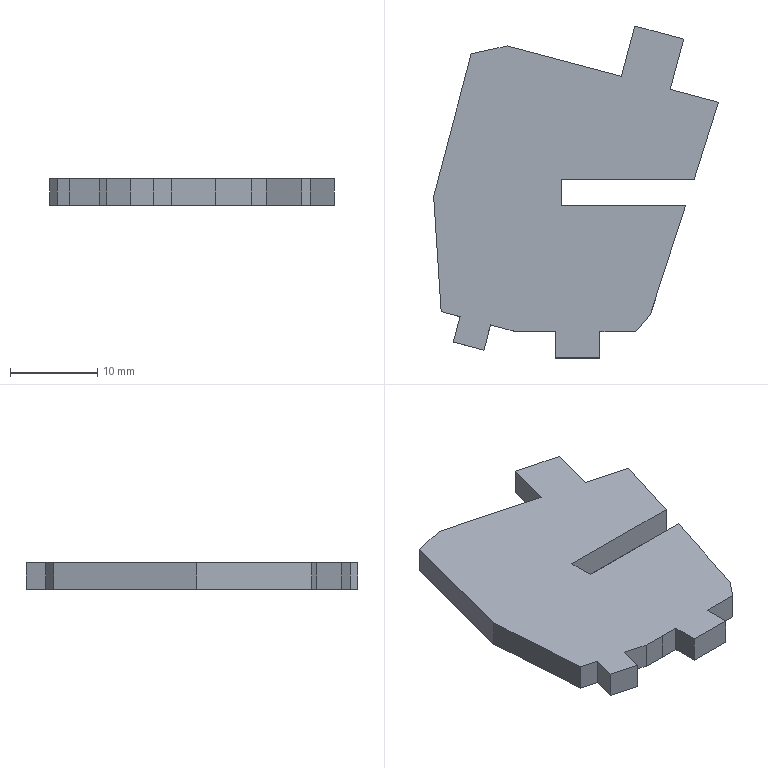Part | SolidWorks | features BaseBody 1 | 1 solid | 27 faces | box 32.712 x 38.137 x 3 mm | volume 2525 mm3 | plane 27
STEP:
#1=CARTESIAN_POINT('',(1.403,4.918,-1.5));
#2=VERTEX_POINT('',#1);
#3=CARTESIAN_POINT('',(16.692,4.918,-1.5));
#4=VERTEX_POINT('',#3);
#5=CARTESIAN_POINT('',(1.403,4.918,-1.5));
#6=DIRECTION('',(1.,0.,0.));
#7=VECTOR('',#6,1000.);
#8=LINE('',#5,#7);
#9=EDGE_CURVE('',#2,#4,#8,.T.);
#10=ORIENTED_EDGE('',*,*,#9,.F.);
#11=CARTESIAN_POINT('',(1.403,1.923,-1.5));
#12=VERTEX_POINT('',#11);
#13=CARTESIAN_POINT('',(1.403,1.923,-1.5));
#14=DIRECTION('',(0.,1.,0.));
#15=VECTOR('',#14,1000.);
#16=LINE('',#13,#15);
#17=EDGE_CURVE('',#12,#2,#16,.T.);
#18=ORIENTED_EDGE('',*,*,#17,.F.);
#19=CARTESIAN_POINT('',(15.72,1.923,-1.5));
#20=VERTEX_POINT('',#19);
#21=CARTESIAN_POINT('',(15.72,1.923,-1.5));
#22=DIRECTION('',(-1.,0.,0.));
#23=VECTOR('',#22,1000.);
#24=LINE('',#21,#23);
#25=EDGE_CURVE('',#20,#12,#24,.T.);
#26=ORIENTED_EDGE('',*,*,#25,.F.);
#27=CARTESIAN_POINT('',(11.682,-10.531,-1.5));
#28=VERTEX_POINT('',#27);
#29=CARTESIAN_POINT('',(11.682,-10.531,-1.5));
#30=DIRECTION('',(0.3085,0.9512,0.));
#31=VECTOR('',#30,1000.);
#32=LINE('',#29,#31);
#33=EDGE_CURVE('',#28,#20,#32,.T.);
#34=ORIENTED_EDGE('',*,*,#33,.F.);
#35=CARTESIAN_POINT('',(9.998,-12.584,-1.5));
#36=VERTEX_POINT('',#35);
#37=CARTESIAN_POINT('',(9.998,-12.584,-1.5));
#38=DIRECTION('',(0.6341,0.7732,0.));
#39=VECTOR('',#38,1000.);
#40=LINE('',#37,#39);
#41=EDGE_CURVE('',#36,#28,#40,.T.);
#42=ORIENTED_EDGE('',*,*,#41,.F.);
#43=CARTESIAN_POINT('',(5.866,-12.584,-1.5));
#44=VERTEX_POINT('',#43);
#45=CARTESIAN_POINT('',(5.866,-12.584,-1.5));
#46=DIRECTION('',(1.,0.,0.));
#47=VECTOR('',#46,1000.);
#48=LINE('',#45,#47);
#49=EDGE_CURVE('',#44,#36,#48,.T.);
#50=ORIENTED_EDGE('',*,*,#49,.F.);
#51=CARTESIAN_POINT('',(5.866,-15.579,-1.5));
#52=VERTEX_POINT('',#51);
#53=CARTESIAN_POINT('',(5.866,-15.579,-1.5));
#54=DIRECTION('',(0.,1.,0.));
#55=VECTOR('',#54,1000.);
#56=LINE('',#53,#55);
#57=EDGE_CURVE('',#52,#44,#56,.T.);
#58=ORIENTED_EDGE('',*,*,#57,.F.);
#59=CARTESIAN_POINT('',(0.8014,-15.579,-1.5));
#60=VERTEX_POINT('',#59);
#61=CARTESIAN_POINT('',(0.8014,-15.579,-1.5));
#62=DIRECTION('',(1.,0.,0.));
#63=VECTOR('',#62,1000.);
#64=LINE('',#61,#63);
#65=EDGE_CURVE('',#60,#52,#64,.T.);
#66=ORIENTED_EDGE('',*,*,#65,.F.);
#67=CARTESIAN_POINT('',(0.8014,-12.584,-1.5));
#68=VERTEX_POINT('',#67);
#69=CARTESIAN_POINT('',(0.8014,-12.584,-1.5));
#70=DIRECTION('',(0.,-1.,0.));
#71=VECTOR('',#70,1000.);
#72=LINE('',#69,#71);
#73=EDGE_CURVE('',#68,#60,#72,.T.);
#74=ORIENTED_EDGE('',*,*,#73,.F.);
#75=CARTESIAN_POINT('',(-1.339,-12.584,-1.5));
#76=VERTEX_POINT('',#75);
#77=CARTESIAN_POINT('',(-1.339,-12.584,-1.5));
#78=DIRECTION('',(1.,0.,0.));
#79=VECTOR('',#78,1000.);
#80=LINE('',#77,#79);
#81=EDGE_CURVE('',#76,#68,#80,.T.);
#82=ORIENTED_EDGE('',*,*,#81,.F.);
#83=CARTESIAN_POINT('',(-3.987,-12.51,-1.5));
#84=VERTEX_POINT('',#83);
#85=CARTESIAN_POINT('',(-3.987,-12.51,-1.5));
#86=DIRECTION('',(0.9996,-0.02815,0.));
#87=VECTOR('',#86,1000.);
#88=LINE('',#85,#87);
#89=EDGE_CURVE('',#84,#76,#88,.T.);
#90=ORIENTED_EDGE('',*,*,#89,.F.);
#91=CARTESIAN_POINT('',(-6.685,-11.785,-1.5));
#92=VERTEX_POINT('',#91);
#93=CARTESIAN_POINT('',(-6.685,-11.785,-1.5));
#94=DIRECTION('',(0.9658,-0.2593,0.));
#95=VECTOR('',#94,1000.);
#96=LINE('',#93,#95);
#97=EDGE_CURVE('',#92,#84,#96,.T.);
#98=ORIENTED_EDGE('',*,*,#97,.F.);
#99=CARTESIAN_POINT('',(-7.463,-14.68,-1.5));
#100=VERTEX_POINT('',#99);
#101=CARTESIAN_POINT('',(-7.463,-14.68,-1.5));
#102=DIRECTION('',(0.2595,0.9658,0.));
#103=VECTOR('',#102,1000.);
#104=LINE('',#101,#103);
#105=EDGE_CURVE('',#100,#92,#104,.T.);
#106=ORIENTED_EDGE('',*,*,#105,.F.);
#107=CARTESIAN_POINT('',(-10.961,-13.742,-1.5));
#108=VERTEX_POINT('',#107);
#109=CARTESIAN_POINT('',(-10.961,-13.742,-1.5));
#110=DIRECTION('',(0.9659,-0.2591,0.));
#111=VECTOR('',#110,1000.);
#112=LINE('',#109,#111);
#113=EDGE_CURVE('',#108,#100,#112,.T.);
#114=ORIENTED_EDGE('',*,*,#113,.F.);
#115=CARTESIAN_POINT('',(-10.185,-10.848,-1.5));
#116=VERTEX_POINT('',#115);
#117=CARTESIAN_POINT('',(-10.185,-10.848,-1.5));
#118=DIRECTION('',(-0.2591,-0.9659,0.));
#119=VECTOR('',#118,1000.);
#120=LINE('',#117,#119);
#121=EDGE_CURVE('',#116,#108,#120,.T.);
#122=ORIENTED_EDGE('',*,*,#121,.F.);
#123=CARTESIAN_POINT('',(-12.37,-10.262,-1.5));
#124=VERTEX_POINT('',#123);
#125=CARTESIAN_POINT('',(-12.37,-10.262,-1.5));
#126=DIRECTION('',(0.9659,-0.259,0.));
#127=VECTOR('',#126,1000.);
#128=LINE('',#125,#127);
#129=EDGE_CURVE('',#124,#116,#128,.T.);
#130=ORIENTED_EDGE('',*,*,#129,.F.);
#131=CARTESIAN_POINT('',(-13.232,2.968,-1.5));
#132=VERTEX_POINT('',#131);
#133=CARTESIAN_POINT('',(-13.232,2.968,-1.5));
#134=DIRECTION('',(0.065,-0.9979,0.));
#135=VECTOR('',#134,1000.);
#136=LINE('',#133,#135);
#137=EDGE_CURVE('',#132,#124,#136,.T.);
#138=ORIENTED_EDGE('',*,*,#137,.F.);
#139=CARTESIAN_POINT('',(-8.91,19.377,-1.5));
#140=VERTEX_POINT('',#139);
#141=CARTESIAN_POINT('',(-8.91,19.377,-1.5));
#142=DIRECTION('',(-0.2547,-0.967,0.));
#143=VECTOR('',#142,1000.);
#144=LINE('',#141,#143);
#145=EDGE_CURVE('',#140,#132,#144,.T.);
#146=ORIENTED_EDGE('',*,*,#145,.F.);
#147=CARTESIAN_POINT('',(-4.779,20.266,-1.5));
#148=VERTEX_POINT('',#147);
#149=CARTESIAN_POINT('',(-4.779,20.266,-1.5));
#150=DIRECTION('',(-0.9776,-0.2104,0.));
#151=VECTOR('',#150,1000.);
#152=LINE('',#149,#151);
#153=EDGE_CURVE('',#148,#140,#152,.T.);
#154=ORIENTED_EDGE('',*,*,#153,.F.);
#155=CARTESIAN_POINT('',(8.324,16.769,-1.5));
#156=VERTEX_POINT('',#155);
#157=CARTESIAN_POINT('',(8.324,16.769,-1.5));
#158=DIRECTION('',(-0.9662,0.2578,0.));
#159=VECTOR('',#158,1000.);
#160=LINE('',#157,#159);
#161=EDGE_CURVE('',#156,#148,#160,.T.);
#162=ORIENTED_EDGE('',*,*,#161,.F.);
#163=CARTESIAN_POINT('',(9.87,22.558,-1.5));
#164=VERTEX_POINT('',#163);
#165=CARTESIAN_POINT('',(9.87,22.558,-1.5));
#166=DIRECTION('',(-0.258,-0.9661,0.));
#167=VECTOR('',#166,1000.);
#168=LINE('',#165,#167);
#169=EDGE_CURVE('',#164,#156,#168,.T.);
#170=ORIENTED_EDGE('',*,*,#169,.F.);
#171=CARTESIAN_POINT('',(15.49,21.059,-1.5));
#172=VERTEX_POINT('',#171);
#173=CARTESIAN_POINT('',(15.49,21.059,-1.5));
#174=DIRECTION('',(-0.9662,0.2576,0.));
#175=VECTOR('',#174,1000.);
#176=LINE('',#173,#175);
#177=EDGE_CURVE('',#172,#164,#176,.T.);
#178=ORIENTED_EDGE('',*,*,#177,.F.);
#179=CARTESIAN_POINT('',(13.938,15.27,-1.5));
#180=VERTEX_POINT('',#179);
#181=CARTESIAN_POINT('',(13.938,15.27,-1.5));
#182=DIRECTION('',(0.259,0.9659,0.));
#183=VECTOR('',#182,1000.);
#184=LINE('',#181,#183);
#185=EDGE_CURVE('',#180,#172,#184,.T.);
#186=ORIENTED_EDGE('',*,*,#185,.F.);
#187=CARTESIAN_POINT('',(19.48,13.793,-1.5));
#188=VERTEX_POINT('',#187);
#189=CARTESIAN_POINT('',(19.48,13.793,-1.5));
#190=DIRECTION('',(-0.9662,0.2576,0.));
#191=VECTOR('',#190,1000.);
#192=LINE('',#189,#191);
#193=EDGE_CURVE('',#188,#180,#192,.T.);
#194=ORIENTED_EDGE('',*,*,#193,.F.);
#195=CARTESIAN_POINT('',(16.692,4.918,-1.5));
#196=DIRECTION('',(0.2997,0.954,0.));
#197=VECTOR('',#196,1000.);
#198=LINE('',#195,#197);
#199=EDGE_CURVE('',#4,#188,#198,.T.);
#200=ORIENTED_EDGE('',*,*,#199,.F.);
#201=EDGE_LOOP('',(#10,#18,#26,#34,#42,#50,#58,#66,#74,#82,#90,#98,#106,#114,#122,#130,#138,#146,#154,#162,#170,#178,#186,#194,#200));
#202=FACE_OUTER_BOUND('',#201,.T.);
#203=CARTESIAN_POINT('',(0.,0.,-1.5));
#204=DIRECTION('',(0.,0.,-1.));
#205=DIRECTION('',(0.,-1.,0.));
#206=AXIS2_PLACEMENT_3D('',#203,#204,#205);
#207=PLANE('',#206);
#208=ADVANCED_FACE('',(#202),#207,.T.);
#209=CARTESIAN_POINT('',(1.403,4.918,1.5));
#210=VERTEX_POINT('',#209);
#211=CARTESIAN_POINT('',(16.692,4.918,1.5));
#212=VERTEX_POINT('',#211);
#213=CARTESIAN_POINT('',(1.403,4.918,1.5));
#214=DIRECTION('',(1.,0.,0.));
#215=VECTOR('',#214,1000.);
#216=LINE('',#213,#215);
#217=EDGE_CURVE('',#210,#212,#216,.T.);
#218=ORIENTED_EDGE('',*,*,#217,.T.);
#219=CARTESIAN_POINT('',(19.48,13.793,1.5));
#220=VERTEX_POINT('',#219);
#221=CARTESIAN_POINT('',(16.692,4.918,1.5));
#222=DIRECTION('',(0.2997,0.954,0.));
#223=VECTOR('',#222,1000.);
#224=LINE('',#221,#223);
#225=EDGE_CURVE('',#212,#220,#224,.T.);
#226=ORIENTED_EDGE('',*,*,#225,.T.);
#227=CARTESIAN_POINT('',(13.938,15.27,1.5));
#228=VERTEX_POINT('',#227);
#229=CARTESIAN_POINT('',(19.48,13.793,1.5));
#230=DIRECTION('',(-0.9662,0.2576,0.));
#231=VECTOR('',#230,1000.);
#232=LINE('',#229,#231);
#233=EDGE_CURVE('',#220,#228,#232,.T.);
#234=ORIENTED_EDGE('',*,*,#233,.T.);
#235=CARTESIAN_POINT('',(15.49,21.059,1.5));
#236=VERTEX_POINT('',#235);
#237=CARTESIAN_POINT('',(13.938,15.27,1.5));
#238=DIRECTION('',(0.259,0.9659,0.));
#239=VECTOR('',#238,1000.);
#240=LINE('',#237,#239);
#241=EDGE_CURVE('',#228,#236,#240,.T.);
#242=ORIENTED_EDGE('',*,*,#241,.T.);
#243=CARTESIAN_POINT('',(9.87,22.558,1.5));
#244=VERTEX_POINT('',#243);
#245=CARTESIAN_POINT('',(15.49,21.059,1.5));
#246=DIRECTION('',(-0.9662,0.2576,0.));
#247=VECTOR('',#246,1000.);
#248=LINE('',#245,#247);
#249=EDGE_CURVE('',#236,#244,#248,.T.);
#250=ORIENTED_EDGE('',*,*,#249,.T.);
#251=CARTESIAN_POINT('',(8.324,16.769,1.5));
#252=VERTEX_POINT('',#251);
#253=CARTESIAN_POINT('',(9.87,22.558,1.5));
#254=DIRECTION('',(-0.258,-0.9661,0.));
#255=VECTOR('',#254,1000.);
#256=LINE('',#253,#255);
#257=EDGE_CURVE('',#244,#252,#256,.T.);
#258=ORIENTED_EDGE('',*,*,#257,.T.);
#259=CARTESIAN_POINT('',(-4.779,20.266,1.5));
#260=VERTEX_POINT('',#259);
#261=CARTESIAN_POINT('',(8.324,16.769,1.5));
#262=DIRECTION('',(-0.9662,0.2578,0.));
#263=VECTOR('',#262,1000.);
#264=LINE('',#261,#263);
#265=EDGE_CURVE('',#252,#260,#264,.T.);
#266=ORIENTED_EDGE('',*,*,#265,.T.);
#267=CARTESIAN_POINT('',(-8.91,19.377,1.5));
#268=VERTEX_POINT('',#267);
#269=CARTESIAN_POINT('',(-4.779,20.266,1.5));
#270=DIRECTION('',(-0.9776,-0.2104,0.));
#271=VECTOR('',#270,1000.);
#272=LINE('',#269,#271);
#273=EDGE_CURVE('',#260,#268,#272,.T.);
#274=ORIENTED_EDGE('',*,*,#273,.T.);
#275=CARTESIAN_POINT('',(-13.232,2.968,1.5));
#276=VERTEX_POINT('',#275);
#277=CARTESIAN_POINT('',(-8.91,19.377,1.5));
#278=DIRECTION('',(-0.2547,-0.967,0.));
#279=VECTOR('',#278,1000.);
#280=LINE('',#277,#279);
#281=EDGE_CURVE('',#268,#276,#280,.T.);
#282=ORIENTED_EDGE('',*,*,#281,.T.);
#283=CARTESIAN_POINT('',(-12.37,-10.262,1.5));
#284=VERTEX_POINT('',#283);
#285=CARTESIAN_POINT('',(-13.232,2.968,1.5));
#286=DIRECTION('',(0.065,-0.9979,0.));
#287=VECTOR('',#286,1000.);
#288=LINE('',#285,#287);
#289=EDGE_CURVE('',#276,#284,#288,.T.);
#290=ORIENTED_EDGE('',*,*,#289,.T.);
#291=CARTESIAN_POINT('',(-10.185,-10.848,1.5));
#292=VERTEX_POINT('',#291);
#293=CARTESIAN_POINT('',(-12.37,-10.262,1.5));
#294=DIRECTION('',(0.9659,-0.259,0.));
#295=VECTOR('',#294,1000.);
#296=LINE('',#293,#295);
#297=EDGE_CURVE('',#284,#292,#296,.T.);
#298=ORIENTED_EDGE('',*,*,#297,.T.);
#299=CARTESIAN_POINT('',(-10.961,-13.742,1.5));
#300=VERTEX_POINT('',#299);
#301=CARTESIAN_POINT('',(-10.185,-10.848,1.5));
#302=DIRECTION('',(-0.2591,-0.9659,0.));
#303=VECTOR('',#302,1000.);
#304=LINE('',#301,#303);
#305=EDGE_CURVE('',#292,#300,#304,.T.);
#306=ORIENTED_EDGE('',*,*,#305,.T.);
#307=CARTESIAN_POINT('',(-7.463,-14.68,1.5));
#308=VERTEX_POINT('',#307);
#309=CARTESIAN_POINT('',(-10.961,-13.742,1.5));
#310=DIRECTION('',(0.9659,-0.2591,0.));
#311=VECTOR('',#310,1000.);
#312=LINE('',#309,#311);
#313=EDGE_CURVE('',#300,#308,#312,.T.);
#314=ORIENTED_EDGE('',*,*,#313,.T.);
#315=CARTESIAN_POINT('',(-6.685,-11.785,1.5));
#316=VERTEX_POINT('',#315);
#317=CARTESIAN_POINT('',(-7.463,-14.68,1.5));
#318=DIRECTION('',(0.2595,0.9658,0.));
#319=VECTOR('',#318,1000.);
#320=LINE('',#317,#319);
#321=EDGE_CURVE('',#308,#316,#320,.T.);
#322=ORIENTED_EDGE('',*,*,#321,.T.);
#323=CARTESIAN_POINT('',(-3.987,-12.51,1.5));
#324=VERTEX_POINT('',#323);
#325=CARTESIAN_POINT('',(-6.685,-11.785,1.5));
#326=DIRECTION('',(0.9658,-0.2593,0.));
#327=VECTOR('',#326,1000.);
#328=LINE('',#325,#327);
#329=EDGE_CURVE('',#316,#324,#328,.T.);
#330=ORIENTED_EDGE('',*,*,#329,.T.);
#331=CARTESIAN_POINT('',(-1.339,-12.584,1.5));
#332=VERTEX_POINT('',#331);
#333=CARTESIAN_POINT('',(-3.987,-12.51,1.5));
#334=DIRECTION('',(0.9996,-0.02815,0.));
#335=VECTOR('',#334,1000.);
#336=LINE('',#333,#335);
#337=EDGE_CURVE('',#324,#332,#336,.T.);
#338=ORIENTED_EDGE('',*,*,#337,.T.);
#339=CARTESIAN_POINT('',(0.8014,-12.584,1.5));
#340=VERTEX_POINT('',#339);
#341=CARTESIAN_POINT('',(-1.339,-12.584,1.5));
#342=DIRECTION('',(1.,0.,0.));
#343=VECTOR('',#342,1000.);
#344=LINE('',#341,#343);
#345=EDGE_CURVE('',#332,#340,#344,.T.);
#346=ORIENTED_EDGE('',*,*,#345,.T.);
#347=CARTESIAN_POINT('',(0.8014,-15.579,1.5));
#348=VERTEX_POINT('',#347);
#349=CARTESIAN_POINT('',(0.8014,-12.584,1.5));
#350=DIRECTION('',(0.,-1.,0.));
#351=VECTOR('',#350,1000.);
#352=LINE('',#349,#351);
#353=EDGE_CURVE('',#340,#348,#352,.T.);
#354=ORIENTED_EDGE('',*,*,#353,.T.);
#355=CARTESIAN_POINT('',(5.866,-15.579,1.5));
#356=VERTEX_POINT('',#355);
#357=CARTESIAN_POINT('',(0.8014,-15.579,1.5));
#358=DIRECTION('',(1.,0.,0.));
#359=VECTOR('',#358,1000.);
#360=LINE('',#357,#359);
#361=EDGE_CURVE('',#348,#356,#360,.T.);
#362=ORIENTED_EDGE('',*,*,#361,.T.);
#363=CARTESIAN_POINT('',(5.866,-12.584,1.5));
#364=VERTEX_POINT('',#363);
#365=CARTESIAN_POINT('',(5.866,-15.579,1.5));
#366=DIRECTION('',(0.,1.,0.));
#367=VECTOR('',#366,1000.);
#368=LINE('',#365,#367);
#369=EDGE_CURVE('',#356,#364,#368,.T.);
#370=ORIENTED_EDGE('',*,*,#369,.T.);
#371=CARTESIAN_POINT('',(9.998,-12.584,1.5));
#372=VERTEX_POINT('',#371);
#373=CARTESIAN_POINT('',(5.866,-12.584,1.5));
#374=DIRECTION('',(1.,0.,0.));
#375=VECTOR('',#374,1000.);
#376=LINE('',#373,#375);
#377=EDGE_CURVE('',#364,#372,#376,.T.);
#378=ORIENTED_EDGE('',*,*,#377,.T.);
#379=CARTESIAN_POINT('',(11.682,-10.531,1.5));
#380=VERTEX_POINT('',#379);
#381=CARTESIAN_POINT('',(9.998,-12.584,1.5));
#382=DIRECTION('',(0.6341,0.7732,0.));
#383=VECTOR('',#382,1000.);
#384=LINE('',#381,#383);
#385=EDGE_CURVE('',#372,#380,#384,.T.);
#386=ORIENTED_EDGE('',*,*,#385,.T.);
#387=CARTESIAN_POINT('',(15.72,1.923,1.5));
#388=VERTEX_POINT('',#387);
#389=CARTESIAN_POINT('',(11.682,-10.531,1.5));
#390=DIRECTION('',(0.3085,0.9512,0.));
#391=VECTOR('',#390,1000.);
#392=LINE('',#389,#391);
#393=EDGE_CURVE('',#380,#388,#392,.T.);
#394=ORIENTED_EDGE('',*,*,#393,.T.);
#395=CARTESIAN_POINT('',(1.403,1.923,1.5));
#396=VERTEX_POINT('',#395);
#397=CARTESIAN_POINT('',(15.72,1.923,1.5));
#398=DIRECTION('',(-1.,0.,0.));
#399=VECTOR('',#398,1000.);
#400=LINE('',#397,#399);
#401=EDGE_CURVE('',#388,#396,#400,.T.);
#402=ORIENTED_EDGE('',*,*,#401,.T.);
#403=CARTESIAN_POINT('',(1.403,1.923,1.5));
#404=DIRECTION('',(0.,1.,0.));
#405=VECTOR('',#404,1000.);
#406=LINE('',#403,#405);
#407=EDGE_CURVE('',#396,#210,#406,.T.);
#408=ORIENTED_EDGE('',*,*,#407,.T.);
#409=EDGE_LOOP('',(#218,#226,#234,#242,#250,#258,#266,#274,#282,#290,#298,#306,#314,#322,#330,#338,#346,#354,#362,#370,#378,#386,#394,#402,#408));
#410=FACE_OUTER_BOUND('',#409,.T.);
#411=CARTESIAN_POINT('',(0.,0.,1.5));
#412=DIRECTION('',(0.,0.,-1.));
#413=DIRECTION('',(0.,-1.,0.));
#414=AXIS2_PLACEMENT_3D('',#411,#412,#413);
#415=PLANE('',#414);
#416=ADVANCED_FACE('',(#410),#415,.F.);
#417=ORIENTED_EDGE('',*,*,#17,.T.);
#418=CARTESIAN_POINT('',(1.403,4.918,1.5));
#419=DIRECTION('',(0.,0.,-1.));
#420=VECTOR('',#419,1000.);
#421=LINE('',#418,#420);
#422=EDGE_CURVE('',#210,#2,#421,.T.);
#423=ORIENTED_EDGE('',*,*,#422,.F.);
#424=ORIENTED_EDGE('',*,*,#407,.F.);
#425=CARTESIAN_POINT('',(1.403,1.923,1.5));
#426=DIRECTION('',(0.,0.,-1.));
#427=VECTOR('',#426,1000.);
#428=LINE('',#425,#427);
#429=EDGE_CURVE('',#396,#12,#428,.T.);
#430=ORIENTED_EDGE('',*,*,#429,.T.);
#431=EDGE_LOOP('',(#417,#423,#424,#430));
#432=FACE_OUTER_BOUND('',#431,.T.);
#433=CARTESIAN_POINT('',(1.403,1.923,1.5));
#434=DIRECTION('',(-1.,0.,0.));
#435=DIRECTION('',(0.,0.,1.));
#436=AXIS2_PLACEMENT_3D('',#433,#434,#435);
#437=PLANE('',#436);
#438=ADVANCED_FACE('',(#432),#437,.F.);
#439=ORIENTED_EDGE('',*,*,#25,.T.);
#440=ORIENTED_EDGE('',*,*,#429,.F.);
#441=ORIENTED_EDGE('',*,*,#401,.F.);
#442=CARTESIAN_POINT('',(15.72,1.923,1.5));
#443=DIRECTION('',(0.,0.,-1.));
#444=VECTOR('',#443,1000.);
#445=LINE('',#442,#444);
#446=EDGE_CURVE('',#388,#20,#445,.T.);
#447=ORIENTED_EDGE('',*,*,#446,.T.);
#448=EDGE_LOOP('',(#439,#440,#441,#447));
#449=FACE_OUTER_BOUND('',#448,.T.);
#450=CARTESIAN_POINT('',(15.72,1.923,1.5));
#451=DIRECTION('',(0.,-1.,0.));
#452=DIRECTION('',(0.,0.,-1.));
#453=AXIS2_PLACEMENT_3D('',#450,#451,#452);
#454=PLANE('',#453);
#455=ADVANCED_FACE('',(#449),#454,.F.);
#456=ORIENTED_EDGE('',*,*,#33,.T.);
#457=ORIENTED_EDGE('',*,*,#446,.F.);
#458=ORIENTED_EDGE('',*,*,#393,.F.);
#459=CARTESIAN_POINT('',(11.682,-10.531,1.5));
#460=DIRECTION('',(0.,0.,-1.));
#461=VECTOR('',#460,1000.);
#462=LINE('',#459,#461);
#463=EDGE_CURVE('',#380,#28,#462,.T.);
#464=ORIENTED_EDGE('',*,*,#463,.T.);
#465=EDGE_LOOP('',(#456,#457,#458,#464));
#466=FACE_OUTER_BOUND('',#465,.T.);
#467=CARTESIAN_POINT('',(11.682,-10.531,1.5));
#468=DIRECTION('',(-0.9512,0.3085,0.));
#469=DIRECTION('',(0.,0.,1.));
#470=AXIS2_PLACEMENT_3D('',#467,#468,#469);
#471=PLANE('',#470);
#472=ADVANCED_FACE('',(#466),#471,.F.);
#473=ORIENTED_EDGE('',*,*,#41,.T.);
#474=ORIENTED_EDGE('',*,*,#463,.F.);
#475=ORIENTED_EDGE('',*,*,#385,.F.);
#476=CARTESIAN_POINT('',(9.998,-12.584,1.5));
#477=DIRECTION('',(0.,0.,-1.));
#478=VECTOR('',#477,1000.);
#479=LINE('',#476,#478);
#480=EDGE_CURVE('',#372,#36,#479,.T.);
#481=ORIENTED_EDGE('',*,*,#480,.T.);
#482=EDGE_LOOP('',(#473,#474,#475,#481));
#483=FACE_OUTER_BOUND('',#482,.T.);
#484=CARTESIAN_POINT('',(9.998,-12.584,1.5));
#485=DIRECTION('',(-0.7732,0.6341,0.));
#486=DIRECTION('',(0.,0.,1.));
#487=AXIS2_PLACEMENT_3D('',#484,#485,#486);
#488=PLANE('',#487);
#489=ADVANCED_FACE('',(#483),#488,.F.);
#490=ORIENTED_EDGE('',*,*,#49,.T.);
#491=ORIENTED_EDGE('',*,*,#480,.F.);
#492=ORIENTED_EDGE('',*,*,#377,.F.);
#493=CARTESIAN_POINT('',(5.866,-12.584,1.5));
#494=DIRECTION('',(0.,0.,-1.));
#495=VECTOR('',#494,1000.);
#496=LINE('',#493,#495);
#497=EDGE_CURVE('',#364,#44,#496,.T.);
#498=ORIENTED_EDGE('',*,*,#497,.T.);
#499=EDGE_LOOP('',(#490,#491,#492,#498));
#500=FACE_OUTER_BOUND('',#499,.T.);
#501=CARTESIAN_POINT('',(5.866,-12.584,1.5));
#502=DIRECTION('',(0.,1.,0.));
#503=DIRECTION('',(1.,0.,0.));
#504=AXIS2_PLACEMENT_3D('',#501,#502,#503);
#505=PLANE('',#504);
#506=ADVANCED_FACE('',(#500),#505,.F.);
#507=ORIENTED_EDGE('',*,*,#57,.T.);
#508=ORIENTED_EDGE('',*,*,#497,.F.);
#509=ORIENTED_EDGE('',*,*,#369,.F.);
#510=CARTESIAN_POINT('',(5.866,-15.579,1.5));
#511=DIRECTION('',(0.,0.,-1.));
#512=VECTOR('',#511,1000.);
#513=LINE('',#510,#512);
#514=EDGE_CURVE('',#356,#52,#513,.T.);
#515=ORIENTED_EDGE('',*,*,#514,.T.);
#516=EDGE_LOOP('',(#507,#508,#509,#515));
#517=FACE_OUTER_BOUND('',#516,.T.);
#518=CARTESIAN_POINT('',(5.866,-15.579,1.5));
#519=DIRECTION('',(-1.,0.,0.));
#520=DIRECTION('',(0.,0.,1.));
#521=AXIS2_PLACEMENT_3D('',#518,#519,#520);
#522=PLANE('',#521);
#523=ADVANCED_FACE('',(#517),#522,.F.);
#524=ORIENTED_EDGE('',*,*,#65,.T.);
#525=ORIENTED_EDGE('',*,*,#514,.F.);
#526=ORIENTED_EDGE('',*,*,#361,.F.);
#527=CARTESIAN_POINT('',(0.8014,-15.579,1.5));
#528=DIRECTION('',(0.,0.,-1.));
#529=VECTOR('',#528,1000.);
#530=LINE('',#527,#529);
#531=EDGE_CURVE('',#348,#60,#530,.T.);
#532=ORIENTED_EDGE('',*,*,#531,.T.);
#533=EDGE_LOOP('',(#524,#525,#526,#532));
#534=FACE_OUTER_BOUND('',#533,.T.);
#535=CARTESIAN_POINT('',(0.8014,-15.579,1.5));
#536=DIRECTION('',(0.,1.,0.));
#537=DIRECTION('',(1.,0.,0.));
#538=AXIS2_PLACEMENT_3D('',#535,#536,#537);
#539=PLANE('',#538);
#540=ADVANCED_FACE('',(#534),#539,.F.);
#541=ORIENTED_EDGE('',*,*,#73,.T.);
#542=ORIENTED_EDGE('',*,*,#531,.F.);
#543=ORIENTED_EDGE('',*,*,#353,.F.);
#544=CARTESIAN_POINT('',(0.8014,-12.584,1.5));
#545=DIRECTION('',(0.,0.,-1.));
#546=VECTOR('',#545,1000.);
#547=LINE('',#544,#546);
#548=EDGE_CURVE('',#340,#68,#547,.T.);
#549=ORIENTED_EDGE('',*,*,#548,.T.);
#550=EDGE_LOOP('',(#541,#542,#543,#549));
#551=FACE_OUTER_BOUND('',#550,.T.);
#552=CARTESIAN_POINT('',(0.8014,-12.584,1.5));
#553=DIRECTION('',(1.,0.,0.));
#554=DIRECTION('',(0.,1.,0.));
#555=AXIS2_PLACEMENT_3D('',#552,#553,#554);
#556=PLANE('',#555);
#557=ADVANCED_FACE('',(#551),#556,.F.);
#558=ORIENTED_EDGE('',*,*,#81,.T.);
#559=ORIENTED_EDGE('',*,*,#548,.F.);
#560=ORIENTED_EDGE('',*,*,#345,.F.);
#561=CARTESIAN_POINT('',(-1.339,-12.584,1.5));
#562=DIRECTION('',(0.,0.,-1.));
#563=VECTOR('',#562,1000.);
#564=LINE('',#561,#563);
#565=EDGE_CURVE('',#332,#76,#564,.T.);
#566=ORIENTED_EDGE('',*,*,#565,.T.);
#567=EDGE_LOOP('',(#558,#559,#560,#566));
#568=FACE_OUTER_BOUND('',#567,.T.);
#569=CARTESIAN_POINT('',(-1.339,-12.584,1.5));
#570=DIRECTION('',(0.,1.,0.));
#571=DIRECTION('',(1.,0.,0.));
#572=AXIS2_PLACEMENT_3D('',#569,#570,#571);
#573=PLANE('',#572);
#574=ADVANCED_FACE('',(#568),#573,.F.);
#575=ORIENTED_EDGE('',*,*,#89,.T.);
#576=ORIENTED_EDGE('',*,*,#565,.F.);
#577=ORIENTED_EDGE('',*,*,#337,.F.);
#578=CARTESIAN_POINT('',(-3.987,-12.51,1.5));
#579=DIRECTION('',(0.,0.,-1.));
#580=VECTOR('',#579,1000.);
#581=LINE('',#578,#580);
#582=EDGE_CURVE('',#324,#84,#581,.T.);
#583=ORIENTED_EDGE('',*,*,#582,.T.);
#584=EDGE_LOOP('',(#575,#576,#577,#583));
#585=FACE_OUTER_BOUND('',#584,.T.);
#586=CARTESIAN_POINT('',(-3.987,-12.51,1.5));
#587=DIRECTION('',(0.02815,0.9996,0.));
#588=DIRECTION('',(0.,0.,-1.));
#589=AXIS2_PLACEMENT_3D('',#586,#587,#588);
#590=PLANE('',#589);
#591=ADVANCED_FACE('',(#585),#590,.F.);
#592=ORIENTED_EDGE('',*,*,#97,.T.);
#593=ORIENTED_EDGE('',*,*,#582,.F.);
#594=ORIENTED_EDGE('',*,*,#329,.F.);
#595=CARTESIAN_POINT('',(-6.685,-11.785,1.5));
#596=DIRECTION('',(0.,0.,-1.));
#597=VECTOR('',#596,1000.);
#598=LINE('',#595,#597);
#599=EDGE_CURVE('',#316,#92,#598,.T.);
#600=ORIENTED_EDGE('',*,*,#599,.T.);
#601=EDGE_LOOP('',(#592,#593,#594,#600));
#602=FACE_OUTER_BOUND('',#601,.T.);
#603=CARTESIAN_POINT('',(-6.685,-11.785,1.5));
#604=DIRECTION('',(0.2593,0.9658,0.));
#605=DIRECTION('',(0.,0.,-1.));
#606=AXIS2_PLACEMENT_3D('',#603,#604,#605);
#607=PLANE('',#606);
#608=ADVANCED_FACE('',(#602),#607,.F.);
#609=ORIENTED_EDGE('',*,*,#105,.T.);
#610=ORIENTED_EDGE('',*,*,#599,.F.);
#611=ORIENTED_EDGE('',*,*,#321,.F.);
#612=CARTESIAN_POINT('',(-7.463,-14.68,1.5));
#613=DIRECTION('',(0.,0.,-1.));
#614=VECTOR('',#613,1000.);
#615=LINE('',#612,#614);
#616=EDGE_CURVE('',#308,#100,#615,.T.);
#617=ORIENTED_EDGE('',*,*,#616,.T.);
#618=EDGE_LOOP('',(#609,#610,#611,#617));
#619=FACE_OUTER_BOUND('',#618,.T.);
#620=CARTESIAN_POINT('',(-7.463,-14.68,1.5));
#621=DIRECTION('',(-0.9658,0.2595,0.));
#622=DIRECTION('',(0.,0.,1.));
#623=AXIS2_PLACEMENT_3D('',#620,#621,#622);
#624=PLANE('',#623);
#625=ADVANCED_FACE('',(#619),#624,.F.);
#626=ORIENTED_EDGE('',*,*,#113,.T.);
#627=ORIENTED_EDGE('',*,*,#616,.F.);
#628=ORIENTED_EDGE('',*,*,#313,.F.);
#629=CARTESIAN_POINT('',(-10.961,-13.742,1.5));
#630=DIRECTION('',(0.,0.,-1.));
#631=VECTOR('',#630,1000.);
#632=LINE('',#629,#631);
#633=EDGE_CURVE('',#300,#108,#632,.T.);
#634=ORIENTED_EDGE('',*,*,#633,.T.);
#635=EDGE_LOOP('',(#626,#627,#628,#634));
#636=FACE_OUTER_BOUND('',#635,.T.);
#637=CARTESIAN_POINT('',(-10.961,-13.742,1.5));
#638=DIRECTION('',(0.2591,0.9659,0.));
#639=DIRECTION('',(0.,0.,-1.));
#640=AXIS2_PLACEMENT_3D('',#637,#638,#639);
#641=PLANE('',#640);
#642=ADVANCED_FACE('',(#636),#641,.F.);
#643=ORIENTED_EDGE('',*,*,#121,.T.);
#644=ORIENTED_EDGE('',*,*,#633,.F.);
#645=ORIENTED_EDGE('',*,*,#305,.F.);
#646=CARTESIAN_POINT('',(-10.185,-10.848,1.5));
#647=DIRECTION('',(0.,0.,-1.));
#648=VECTOR('',#647,1000.);
#649=LINE('',#646,#648);
#650=EDGE_CURVE('',#292,#116,#649,.T.);
#651=ORIENTED_EDGE('',*,*,#650,.T.);
#652=EDGE_LOOP('',(#643,#644,#645,#651));
#653=FACE_OUTER_BOUND('',#652,.T.);
#654=CARTESIAN_POINT('',(-10.185,-10.848,1.5));
#655=DIRECTION('',(0.9659,-0.2591,0.));
#656=DIRECTION('',(0.,0.,-1.));
#657=AXIS2_PLACEMENT_3D('',#654,#655,#656);
#658=PLANE('',#657);
#659=ADVANCED_FACE('',(#653),#658,.F.);
#660=ORIENTED_EDGE('',*,*,#129,.T.);
#661=ORIENTED_EDGE('',*,*,#650,.F.);
#662=ORIENTED_EDGE('',*,*,#297,.F.);
#663=CARTESIAN_POINT('',(-12.37,-10.262,1.5));
#664=DIRECTION('',(0.,0.,-1.));
#665=VECTOR('',#664,1000.);
#666=LINE('',#663,#665);
#667=EDGE_CURVE('',#284,#124,#666,.T.);
#668=ORIENTED_EDGE('',*,*,#667,.T.);
#669=EDGE_LOOP('',(#660,#661,#662,#668));
#670=FACE_OUTER_BOUND('',#669,.T.);
#671=CARTESIAN_POINT('',(-12.37,-10.262,1.5));
#672=DIRECTION('',(0.259,0.9659,0.));
#673=DIRECTION('',(0.,0.,-1.));
#674=AXIS2_PLACEMENT_3D('',#671,#672,#673);
#675=PLANE('',#674);
#676=ADVANCED_FACE('',(#670),#675,.F.);
#677=ORIENTED_EDGE('',*,*,#137,.T.);
#678=ORIENTED_EDGE('',*,*,#667,.F.);
#679=ORIENTED_EDGE('',*,*,#289,.F.);
#680=CARTESIAN_POINT('',(-13.232,2.968,1.5));
#681=DIRECTION('',(0.,0.,-1.));
#682=VECTOR('',#681,1000.);
#683=LINE('',#680,#682);
#684=EDGE_CURVE('',#276,#132,#683,.T.);
#685=ORIENTED_EDGE('',*,*,#684,.T.);
#686=EDGE_LOOP('',(#677,#678,#679,#685));
#687=FACE_OUTER_BOUND('',#686,.T.);
#688=CARTESIAN_POINT('',(-13.232,2.968,1.5));
#689=DIRECTION('',(0.9979,0.065,0.));
#690=DIRECTION('',(0.,0.,-1.));
#691=AXIS2_PLACEMENT_3D('',#688,#689,#690);
#692=PLANE('',#691);
#693=ADVANCED_FACE('',(#687),#692,.F.);
#694=ORIENTED_EDGE('',*,*,#145,.T.);
#695=ORIENTED_EDGE('',*,*,#684,.F.);
#696=ORIENTED_EDGE('',*,*,#281,.F.);
#697=CARTESIAN_POINT('',(-8.91,19.377,1.5));
#698=DIRECTION('',(0.,0.,-1.));
#699=VECTOR('',#698,1000.);
#700=LINE('',#697,#699);
#701=EDGE_CURVE('',#268,#140,#700,.T.);
#702=ORIENTED_EDGE('',*,*,#701,.T.);
#703=EDGE_LOOP('',(#694,#695,#696,#702));
#704=FACE_OUTER_BOUND('',#703,.T.);
#705=CARTESIAN_POINT('',(-8.91,19.377,1.5));
#706=DIRECTION('',(0.967,-0.2547,0.));
#707=DIRECTION('',(0.,0.,-1.));
#708=AXIS2_PLACEMENT_3D('',#705,#706,#707);
#709=PLANE('',#708);
#710=ADVANCED_FACE('',(#704),#709,.F.);
#711=ORIENTED_EDGE('',*,*,#153,.T.);
#712=ORIENTED_EDGE('',*,*,#701,.F.);
#713=ORIENTED_EDGE('',*,*,#273,.F.);
#714=CARTESIAN_POINT('',(-4.779,20.266,1.5));
#715=DIRECTION('',(0.,0.,-1.));
#716=VECTOR('',#715,1000.);
#717=LINE('',#714,#716);
#718=EDGE_CURVE('',#260,#148,#717,.T.);
#719=ORIENTED_EDGE('',*,*,#718,.T.);
#720=EDGE_LOOP('',(#711,#712,#713,#719));
#721=FACE_OUTER_BOUND('',#720,.T.);
#722=CARTESIAN_POINT('',(-4.779,20.266,1.5));
#723=DIRECTION('',(0.2104,-0.9776,0.));
#724=DIRECTION('',(0.,0.,-1.));
#725=AXIS2_PLACEMENT_3D('',#722,#723,#724);
#726=PLANE('',#725);
#727=ADVANCED_FACE('',(#721),#726,.F.);
#728=ORIENTED_EDGE('',*,*,#161,.T.);
#729=ORIENTED_EDGE('',*,*,#718,.F.);
#730=ORIENTED_EDGE('',*,*,#265,.F.);
#731=CARTESIAN_POINT('',(8.324,16.769,1.5));
#732=DIRECTION('',(0.,0.,-1.));
#733=VECTOR('',#732,1000.);
#734=LINE('',#731,#733);
#735=EDGE_CURVE('',#252,#156,#734,.T.);
#736=ORIENTED_EDGE('',*,*,#735,.T.);
#737=EDGE_LOOP('',(#728,#729,#730,#736));
#738=FACE_OUTER_BOUND('',#737,.T.);
#739=CARTESIAN_POINT('',(8.324,16.769,1.5));
#740=DIRECTION('',(-0.2578,-0.9662,0.));
#741=DIRECTION('',(-0.9662,0.2578,0.));
#742=AXIS2_PLACEMENT_3D('',#739,#740,#741);
#743=PLANE('',#742);
#744=ADVANCED_FACE('',(#738),#743,.F.);
#745=ORIENTED_EDGE('',*,*,#169,.T.);
#746=ORIENTED_EDGE('',*,*,#735,.F.);
#747=ORIENTED_EDGE('',*,*,#257,.F.);
#748=CARTESIAN_POINT('',(9.87,22.558,1.5));
#749=DIRECTION('',(0.,0.,-1.));
#750=VECTOR('',#749,1000.);
#751=LINE('',#748,#750);
#752=EDGE_CURVE('',#244,#164,#751,.T.);
#753=ORIENTED_EDGE('',*,*,#752,.T.);
#754=EDGE_LOOP('',(#745,#746,#747,#753));
#755=FACE_OUTER_BOUND('',#754,.T.);
#756=CARTESIAN_POINT('',(9.87,22.558,1.5));
#757=DIRECTION('',(0.9661,-0.258,0.));
#758=DIRECTION('',(0.,0.,-1.));
#759=AXIS2_PLACEMENT_3D('',#756,#757,#758);
#760=PLANE('',#759);
#761=ADVANCED_FACE('',(#755),#760,.F.);
#762=ORIENTED_EDGE('',*,*,#177,.T.);
#763=ORIENTED_EDGE('',*,*,#752,.F.);
#764=ORIENTED_EDGE('',*,*,#249,.F.);
#765=CARTESIAN_POINT('',(15.49,21.059,1.5));
#766=DIRECTION('',(0.,0.,-1.));
#767=VECTOR('',#766,1000.);
#768=LINE('',#765,#767);
#769=EDGE_CURVE('',#236,#172,#768,.T.);
#770=ORIENTED_EDGE('',*,*,#769,.T.);
#771=EDGE_LOOP('',(#762,#763,#764,#770));
#772=FACE_OUTER_BOUND('',#771,.T.);
#773=CARTESIAN_POINT('',(15.49,21.059,1.5));
#774=DIRECTION('',(-0.2576,-0.9662,0.));
#775=DIRECTION('',(-0.9662,0.2576,0.));
#776=AXIS2_PLACEMENT_3D('',#773,#774,#775);
#777=PLANE('',#776);
#778=ADVANCED_FACE('',(#772),#777,.F.);
#779=ORIENTED_EDGE('',*,*,#185,.T.);
#780=ORIENTED_EDGE('',*,*,#769,.F.);
#781=ORIENTED_EDGE('',*,*,#241,.F.);
#782=CARTESIAN_POINT('',(13.938,15.27,1.5));
#783=DIRECTION('',(0.,0.,-1.));
#784=VECTOR('',#783,1000.);
#785=LINE('',#782,#784);
#786=EDGE_CURVE('',#228,#180,#785,.T.);
#787=ORIENTED_EDGE('',*,*,#786,.T.);
#788=EDGE_LOOP('',(#779,#780,#781,#787));
#789=FACE_OUTER_BOUND('',#788,.T.);
#790=CARTESIAN_POINT('',(13.938,15.27,1.5));
#791=DIRECTION('',(-0.9659,0.259,0.));
#792=DIRECTION('',(0.,0.,1.));
#793=AXIS2_PLACEMENT_3D('',#790,#791,#792);
#794=PLANE('',#793);
#795=ADVANCED_FACE('',(#789),#794,.F.);
#796=ORIENTED_EDGE('',*,*,#193,.T.);
#797=ORIENTED_EDGE('',*,*,#786,.F.);
#798=ORIENTED_EDGE('',*,*,#233,.F.);
#799=CARTESIAN_POINT('',(19.48,13.793,1.5));
#800=DIRECTION('',(0.,0.,-1.));
#801=VECTOR('',#800,1000.);
#802=LINE('',#799,#801);
#803=EDGE_CURVE('',#220,#188,#802,.T.);
#804=ORIENTED_EDGE('',*,*,#803,.T.);
#805=EDGE_LOOP('',(#796,#797,#798,#804));
#806=FACE_OUTER_BOUND('',#805,.T.);
#807=CARTESIAN_POINT('',(19.48,13.793,1.5));
#808=DIRECTION('',(-0.2576,-0.9662,0.));
#809=DIRECTION('',(-0.9662,0.2576,0.));
#810=AXIS2_PLACEMENT_3D('',#807,#808,#809);
#811=PLANE('',#810);
#812=ADVANCED_FACE('',(#806),#811,.F.);
#813=ORIENTED_EDGE('',*,*,#199,.T.);
#814=ORIENTED_EDGE('',*,*,#803,.F.);
#815=ORIENTED_EDGE('',*,*,#225,.F.);
#816=CARTESIAN_POINT('',(16.692,4.918,1.5));
#817=DIRECTION('',(0.,0.,-1.));
#818=VECTOR('',#817,1000.);
#819=LINE('',#816,#818);
#820=EDGE_CURVE('',#212,#4,#819,.T.);
#821=ORIENTED_EDGE('',*,*,#820,.T.);
#822=EDGE_LOOP('',(#813,#814,#815,#821));
#823=FACE_OUTER_BOUND('',#822,.T.);
#824=CARTESIAN_POINT('',(16.692,4.918,1.5));
#825=DIRECTION('',(-0.954,0.2997,0.));
#826=DIRECTION('',(0.,0.,1.));
#827=AXIS2_PLACEMENT_3D('',#824,#825,#826);
#828=PLANE('',#827);
#829=ADVANCED_FACE('',(#823),#828,.F.);
#830=ORIENTED_EDGE('',*,*,#9,.T.);
#831=ORIENTED_EDGE('',*,*,#820,.F.);
#832=ORIENTED_EDGE('',*,*,#217,.F.);
#833=ORIENTED_EDGE('',*,*,#422,.T.);
#834=EDGE_LOOP('',(#830,#831,#832,#833));
#835=FACE_OUTER_BOUND('',#834,.T.);
#836=CARTESIAN_POINT('',(1.403,4.918,1.5));
#837=DIRECTION('',(0.,1.,0.));
#838=DIRECTION('',(1.,0.,0.));
#839=AXIS2_PLACEMENT_3D('',#836,#837,#838);
#840=PLANE('',#839);
#841=ADVANCED_FACE('',(#835),#840,.F.);
#842=CLOSED_SHELL('',(#208,#416,#438,#455,#472,#489,#506,#523,#540,#557,#574,#591,#608,#625,#642,#659,#676,#693,#710,#727,#744,#761,#778,#795,#812,#829,#841));
#843=MANIFOLD_SOLID_BREP('',#842);
#844=CARTESIAN_POINT('',(0.,0.,0.));
#845=DIRECTION('',(0.,0.,1.));
#846=DIRECTION('',(1.,0.,0.));
#847=AXIS2_PLACEMENT_3D('',#844,#845,#846);
#848=(LENGTH_UNIT()NAMED_UNIT(*)SI_UNIT(.MILLI.,.METRE.));
#849=UNCERTAINTY_MEASURE_WITH_UNIT(LENGTH_MEASURE(0.00001),#848,'','');
#850=(NAMED_UNIT(*)PLANE_ANGLE_UNIT()SI_UNIT($,.RADIAN.));
#851=(NAMED_UNIT(*)SI_UNIT($,.STERADIAN.)SOLID_ANGLE_UNIT());
#852=(GEOMETRIC_REPRESENTATION_CONTEXT(3)GLOBAL_UNCERTAINTY_ASSIGNED_CONTEXT((#849))GLOBAL_UNIT_ASSIGNED_CONTEXT((#848,#850,#851))REPRESENTATION_CONTEXT('',''));
#853=ADVANCED_BREP_SHAPE_REPRESENTATION('',(#843,#847),#852);